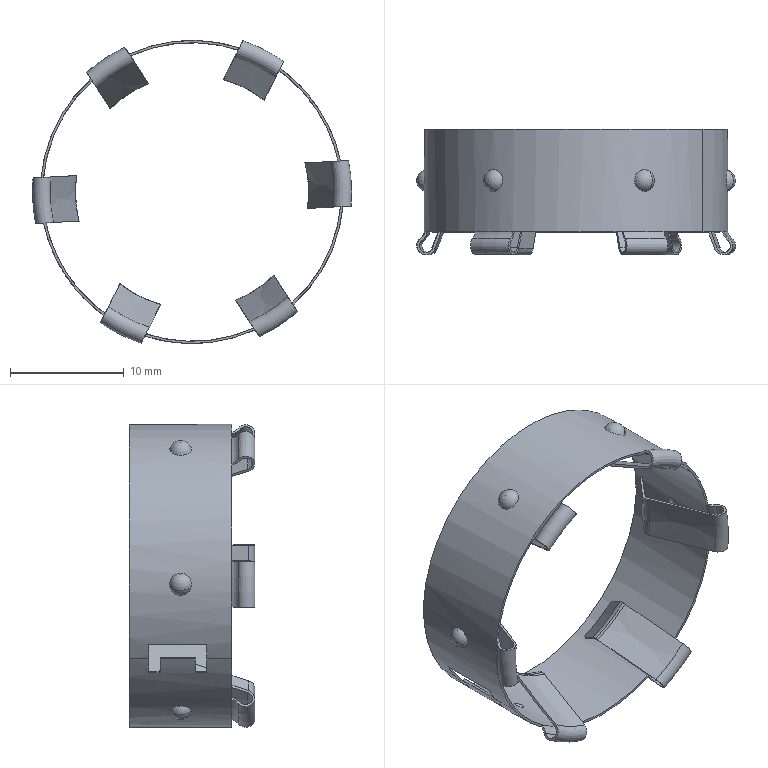Part | SolidWorks | features BaseBody 1 | 1 solid | 153 faces | box 28 x 11 x 26.6 mm | volume 215.957 mm3 | torus 48 | sphere 32 | cone 30 | plane 27 | cylinder 16 | commonest cylinder face diameters 26.6 x8 24.394 x6 26.2 x2